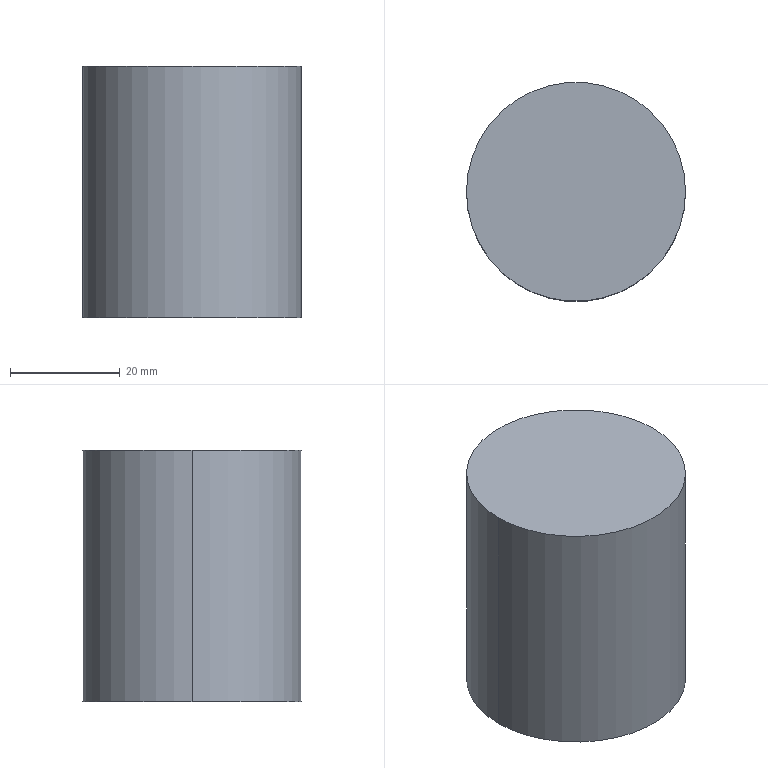Part | SolidWorks | features Extrusion 1 | 1 solid | 4 faces | box 40 x 40 x 46 mm | volume 57805 mm3 | cylinder 2 | plane 2 | commonest cylinder face diameters 40 x2
STEP:
#1=CARTESIAN_POINT('',(141.674,138.644,46.));
#2=VERTEX_POINT('',#1);
#3=CARTESIAN_POINT('',(101.674,138.644,46.));
#4=VERTEX_POINT('',#3);
#5=CARTESIAN_POINT('',(121.674,138.644,46.));
#6=DIRECTION('',(0.,0.,1.));
#7=DIRECTION('',(1.,0.,0.));
#8=AXIS2_PLACEMENT_3D('',#5,#6,#7);
#9=CIRCLE('',#8,20.);
#10=EDGE_CURVE('',#2,#4,#9,.T.);
#11=ORIENTED_EDGE('',*,*,#10,.F.);
#12=CARTESIAN_POINT('',(141.674,138.644,0.));
#13=VERTEX_POINT('',#12);
#14=CARTESIAN_POINT('',(141.674,138.644,46.));
#15=DIRECTION('',(0.,0.,-1.));
#16=VECTOR('',#15,1000.);
#17=LINE('',#14,#16);
#18=EDGE_CURVE('',#2,#13,#17,.T.);
#19=ORIENTED_EDGE('',*,*,#18,.T.);
#20=CARTESIAN_POINT('',(101.674,138.644,0.));
#21=VERTEX_POINT('',#20);
#22=CARTESIAN_POINT('',(121.674,138.644,0.));
#23=DIRECTION('',(0.,0.,1.));
#24=DIRECTION('',(1.,0.,0.));
#25=AXIS2_PLACEMENT_3D('',#22,#23,#24);
#26=CIRCLE('',#25,20.);
#27=EDGE_CURVE('',#13,#21,#26,.T.);
#28=ORIENTED_EDGE('',*,*,#27,.T.);
#29=CARTESIAN_POINT('',(101.674,138.644,46.));
#30=DIRECTION('',(0.,0.,-1.));
#31=VECTOR('',#30,1000.);
#32=LINE('',#29,#31);
#33=EDGE_CURVE('',#4,#21,#32,.T.);
#34=ORIENTED_EDGE('',*,*,#33,.F.);
#35=EDGE_LOOP('',(#11,#19,#28,#34));
#36=FACE_OUTER_BOUND('',#35,.T.);
#37=CARTESIAN_POINT('',(121.674,138.644,46.));
#38=DIRECTION('',(0.,0.,-1.));
#39=DIRECTION('',(-1.,0.,0.));
#40=AXIS2_PLACEMENT_3D('',#37,#38,#39);
#41=CYLINDRICAL_SURFACE('',#40,20.);
#42=ADVANCED_FACE('',(#36),#41,.T.);
#43=ORIENTED_EDGE('',*,*,#18,.F.);
#44=CARTESIAN_POINT('',(121.674,138.644,46.));
#45=DIRECTION('',(0.,0.,1.));
#46=DIRECTION('',(1.,0.,0.));
#47=AXIS2_PLACEMENT_3D('',#44,#45,#46);
#48=CIRCLE('',#47,20.);
#49=EDGE_CURVE('',#4,#2,#48,.T.);
#50=ORIENTED_EDGE('',*,*,#49,.F.);
#51=ORIENTED_EDGE('',*,*,#33,.T.);
#52=CARTESIAN_POINT('',(121.674,138.644,0.));
#53=DIRECTION('',(0.,0.,1.));
#54=DIRECTION('',(1.,0.,0.));
#55=AXIS2_PLACEMENT_3D('',#52,#53,#54);
#56=CIRCLE('',#55,20.);
#57=EDGE_CURVE('',#21,#13,#56,.T.);
#58=ORIENTED_EDGE('',*,*,#57,.T.);
#59=EDGE_LOOP('',(#43,#50,#51,#58));
#60=FACE_OUTER_BOUND('',#59,.T.);
#61=CARTESIAN_POINT('',(121.674,138.644,46.));
#62=DIRECTION('',(0.,0.,-1.));
#63=DIRECTION('',(-1.,0.,0.));
#64=AXIS2_PLACEMENT_3D('',#61,#62,#63);
#65=CYLINDRICAL_SURFACE('',#64,20.);
#66=ADVANCED_FACE('',(#60),#65,.T.);
#67=ORIENTED_EDGE('',*,*,#49,.T.);
#68=ORIENTED_EDGE('',*,*,#10,.T.);
#69=EDGE_LOOP('',(#67,#68));
#70=FACE_OUTER_BOUND('',#69,.T.);
#71=CARTESIAN_POINT('',(121.674,138.644,46.));
#72=DIRECTION('',(0.,0.,1.));
#73=DIRECTION('',(1.,0.,0.));
#74=AXIS2_PLACEMENT_3D('',#71,#72,#73);
#75=PLANE('',#74);
#76=ADVANCED_FACE('',(#70),#75,.T.);
#77=ORIENTED_EDGE('',*,*,#57,.F.);
#78=ORIENTED_EDGE('',*,*,#27,.F.);
#79=EDGE_LOOP('',(#77,#78));
#80=FACE_OUTER_BOUND('',#79,.T.);
#81=CARTESIAN_POINT('',(121.674,138.644,0.));
#82=DIRECTION('',(0.,0.,1.));
#83=DIRECTION('',(1.,0.,0.));
#84=AXIS2_PLACEMENT_3D('',#81,#82,#83);
#85=PLANE('',#84);
#86=ADVANCED_FACE('',(#80),#85,.F.);
#87=CLOSED_SHELL('',(#42,#66,#76,#86));
#88=MANIFOLD_SOLID_BREP('',#87);
#89=CARTESIAN_POINT('',(0.,0.,0.));
#90=DIRECTION('',(0.,0.,1.));
#91=DIRECTION('',(1.,0.,0.));
#92=AXIS2_PLACEMENT_3D('',#89,#90,#91);
#93=(LENGTH_UNIT()NAMED_UNIT(*)SI_UNIT(.MILLI.,.METRE.));
#94=UNCERTAINTY_MEASURE_WITH_UNIT(LENGTH_MEASURE(0.00001),#93,'','');
#95=(NAMED_UNIT(*)PLANE_ANGLE_UNIT()SI_UNIT($,.RADIAN.));
#96=(NAMED_UNIT(*)SI_UNIT($,.STERADIAN.)SOLID_ANGLE_UNIT());
#97=(GEOMETRIC_REPRESENTATION_CONTEXT(3)GLOBAL_UNCERTAINTY_ASSIGNED_CONTEXT((#94))GLOBAL_UNIT_ASSIGNED_CONTEXT((#93,#95,#96))REPRESENTATION_CONTEXT('',''));
#98=ADVANCED_BREP_SHAPE_REPRESENTATION('',(#88,#92),#97);